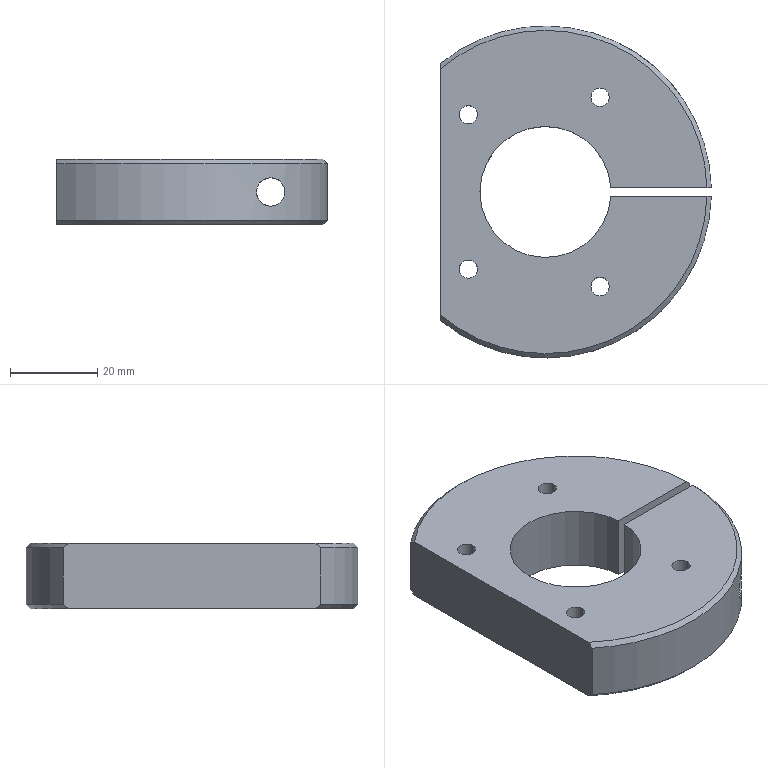Part | SolidWorks | features HoleWzd 3, Chamfer 1, Extrusion 1, ICE 1, RevCut 1 | 1 solid | 28 faces | box 61.987 x 76 x 15 mm | volume 44061 mm3 | cylinder 18 | plane 6 | cone 4 | commonest cylinder face diameters 4.2 x8 6.5 x4 11 x2 30 x2 76 x2
STEP:
#1=CARTESIAN_POINT('',(25.,-28.618,3.25));
#2=VERTEX_POINT('',#1);
#3=CARTESIAN_POINT('',(25.,-28.618,-3.25));
#4=VERTEX_POINT('',#3);
#5=CARTESIAN_POINT('',(25.,-28.618,3.25));
#6=CARTESIAN_POINT('',(24.632,-28.94,3.25));
#7=CARTESIAN_POINT('',(24.265,-29.248,3.189));
#8=CARTESIAN_POINT('',(23.719,-29.69,2.993));
#9=CARTESIAN_POINT('',(23.538,-29.833,2.91));
#10=CARTESIAN_POINT('',(23.192,-30.103,2.708));
#11=CARTESIAN_POINT('',(23.024,-30.231,2.589));
#12=CARTESIAN_POINT('',(22.704,-30.472,2.31));
#13=CARTESIAN_POINT('',(22.554,-30.583,2.152));
#14=CARTESIAN_POINT('',(22.285,-30.78,1.8));
#15=CARTESIAN_POINT('',(22.164,-30.867,1.604));
#16=CARTESIAN_POINT('',(21.965,-31.009,1.184));
#17=CARTESIAN_POINT('',(21.887,-31.064,0.9629));
#18=CARTESIAN_POINT('',(21.806,-31.121,0.6114));
#19=CARTESIAN_POINT('',(21.785,-31.135,0.4903));
#20=CARTESIAN_POINT('',(21.757,-31.155,0.2493));
#21=CARTESIAN_POINT('',(21.75,-31.16,0.1285));
#22=CARTESIAN_POINT('',(21.749,-31.16,-0.2346));
#23=CARTESIAN_POINT('',(21.777,-31.141,-0.481));
#24=CARTESIAN_POINT('',(21.883,-31.067,-0.9495));
#25=CARTESIAN_POINT('',(21.961,-31.012,-1.176));
#26=CARTESIAN_POINT('',(22.161,-30.869,-1.599));
#27=CARTESIAN_POINT('',(22.28,-30.784,-1.793));
#28=CARTESIAN_POINT('',(22.551,-30.585,-2.149));
#29=CARTESIAN_POINT('',(22.701,-30.475,-2.307));
#30=CARTESIAN_POINT('',(23.02,-30.235,-2.586));
#31=CARTESIAN_POINT('',(23.19,-30.104,-2.707));
#32=CARTESIAN_POINT('',(23.538,-29.833,-2.91));
#33=CARTESIAN_POINT('',(23.716,-29.692,-2.992));
#34=CARTESIAN_POINT('',(24.079,-29.399,-3.123));
#35=CARTESIAN_POINT('',(24.265,-29.245,-3.171));
#36=CARTESIAN_POINT('',(24.634,-28.935,-3.235));
#37=CARTESIAN_POINT('',(24.817,-28.778,-3.25));
#38=CARTESIAN_POINT('',(25.,-28.618,-3.25));
#39=B_SPLINE_CURVE_WITH_KNOTS('',3,(#5,#6,#7,#8,#9,#10,#11,#12,#13,#14,#15,#16,#17,#18,#19,#20,#21,#22,#23,#24,#25,#26,#27,#28,#29,#30,#31,#32,#33,#34,#35,#36,#37,#38),.UNSPECIFIED.,.F.,.F.,(4,2,2,2,2,2,2,2,2,2,2,2,2,2,2,2,4),(0.,0.001448,0.002172,0.002897,0.003621,0.004345,0.005069,0.005431,0.005793,0.006517,0.007241,0.007966,0.00869,0.009414,0.01014,0.01086,0.01159),.UNSPECIFIED.);
#40=EDGE_CURVE('',#2,#4,#39,.T.);
#41=ORIENTED_EDGE('',*,*,#40,.T.);
#42=CARTESIAN_POINT('',(25.,-1.,-3.25));
#43=VERTEX_POINT('',#42);
#44=CARTESIAN_POINT('',(25.,32.615,-3.25));
#45=DIRECTION('',(0.,1.,0.));
#46=VECTOR('',#45,1000.);
#47=LINE('',#44,#46);
#48=EDGE_CURVE('',#4,#43,#47,.T.);
#49=ORIENTED_EDGE('',*,*,#48,.T.);
#50=CARTESIAN_POINT('',(25.,-1.,3.25));
#51=VERTEX_POINT('',#50);
#52=CARTESIAN_POINT('',(25.,-1.,0.));
#53=DIRECTION('',(0.,-1.,0.));
#54=DIRECTION('',(1.,0.,0.));
#55=AXIS2_PLACEMENT_3D('',#52,#53,#54);
#56=CIRCLE('',#55,3.25);
#57=EDGE_CURVE('',#51,#43,#56,.T.);
#58=ORIENTED_EDGE('',*,*,#57,.F.);
#59=CARTESIAN_POINT('',(25.,32.615,3.25));
#60=DIRECTION('',(0.,1.,0.));
#61=VECTOR('',#60,1000.);
#62=LINE('',#59,#61);
#63=EDGE_CURVE('',#2,#51,#62,.T.);
#64=ORIENTED_EDGE('',*,*,#63,.F.);
#65=EDGE_LOOP('',(#41,#49,#58,#64));
#66=FACE_OUTER_BOUND('',#65,.T.);
#67=CARTESIAN_POINT('',(25.,32.615,0.));
#68=DIRECTION('',(0.,1.,0.));
#69=DIRECTION('',(0.,0.,1.));
#70=AXIS2_PLACEMENT_3D('',#67,#68,#69);
#71=CYLINDRICAL_SURFACE('',#70,3.25);
#72=ADVANCED_FACE('',(#66),#71,.F.);
#73=CARTESIAN_POINT('',(25.,8.,-5.5));
#74=VERTEX_POINT('',#73);
#75=CARTESIAN_POINT('',(25.,8.,5.5));
#76=VERTEX_POINT('',#75);
#77=CARTESIAN_POINT('',(25.,8.,0.));
#78=DIRECTION('',(0.,1.,0.));
#79=DIRECTION('',(0.,0.,1.));
#80=AXIS2_PLACEMENT_3D('',#77,#78,#79);
#81=CIRCLE('',#80,5.5);
#82=EDGE_CURVE('',#74,#76,#81,.T.);
#83=ORIENTED_EDGE('',*,*,#82,.F.);
#84=CARTESIAN_POINT('',(25.,28.618,-5.5));
#85=VERTEX_POINT('',#84);
#86=CARTESIAN_POINT('',(25.,32.615,-5.5));
#87=DIRECTION('',(0.,1.,0.));
#88=VECTOR('',#87,1000.);
#89=LINE('',#86,#88);
#90=EDGE_CURVE('',#74,#85,#89,.T.);
#91=ORIENTED_EDGE('',*,*,#90,.T.);
#92=CARTESIAN_POINT('',(25.,28.618,5.5));
#93=VERTEX_POINT('',#92);
#94=CARTESIAN_POINT('',(25.,28.618,-5.5));
#95=CARTESIAN_POINT('',(24.694,28.886,-5.5));
#96=CARTESIAN_POINT('',(24.384,29.148,-5.474));
#97=CARTESIAN_POINT('',(23.766,29.654,-5.369));
#98=CARTESIAN_POINT('',(23.457,29.899,-5.289));
#99=CARTESIAN_POINT('',(22.838,30.374,-5.068));
#100=CARTESIAN_POINT('',(22.529,30.603,-4.926));
#101=CARTESIAN_POINT('',(21.937,31.031,-4.581));
#102=CARTESIAN_POINT('',(21.651,31.23,-4.378));
#103=CARTESIAN_POINT('',(21.242,31.509,-4.02));
#104=CARTESIAN_POINT('',(21.109,31.598,-3.892));
#105=CARTESIAN_POINT('',(20.857,31.765,-3.622));
#106=CARTESIAN_POINT('',(20.736,31.844,-3.479));
#107=CARTESIAN_POINT('',(20.509,31.991,-3.18));
#108=CARTESIAN_POINT('',(20.401,32.059,-3.023));
#109=CARTESIAN_POINT('',(20.2,32.186,-2.692));
#110=CARTESIAN_POINT('',(20.107,32.245,-2.519));
#111=CARTESIAN_POINT('',(19.857,32.4,-1.987));
#112=CARTESIAN_POINT('',(19.727,32.479,-1.614));
#113=CARTESIAN_POINT('',(19.593,32.56,-1.025));
#114=CARTESIAN_POINT('',(19.558,32.58,-0.8225));
#115=CARTESIAN_POINT('',(19.512,32.608,-0.4199));
#116=CARTESIAN_POINT('',(19.501,32.615,-0.2183));
#117=CARTESIAN_POINT('',(19.499,32.616,0.1856));
#118=CARTESIAN_POINT('',(19.51,32.609,0.3879));
#119=CARTESIAN_POINT('',(19.554,32.583,0.7932));
#120=CARTESIAN_POINT('',(19.587,32.563,0.9947));
#121=CARTESIAN_POINT('',(19.674,32.511,1.387));
#122=CARTESIAN_POINT('',(19.728,32.478,1.579));
#123=CARTESIAN_POINT('',(19.856,32.4,1.956));
#124=CARTESIAN_POINT('',(19.93,32.354,2.142));
#125=CARTESIAN_POINT('',(20.18,32.199,2.679));
#126=CARTESIAN_POINT('',(20.38,32.074,3.008));
#127=CARTESIAN_POINT('',(20.723,31.853,3.463));
#128=CARTESIAN_POINT('',(20.845,31.773,3.608));
#129=CARTESIAN_POINT('',(21.097,31.606,3.88));
#130=CARTESIAN_POINT('',(21.228,31.518,4.007));
#131=CARTESIAN_POINT('',(21.634,31.242,4.365));
#132=CARTESIAN_POINT('',(21.925,31.039,4.573));
#133=CARTESIAN_POINT('',(22.52,30.61,4.921));
#134=CARTESIAN_POINT('',(22.825,30.384,5.062));
#135=CARTESIAN_POINT('',(23.445,29.908,5.286));
#136=CARTESIAN_POINT('',(23.76,29.659,5.368));
#137=CARTESIAN_POINT('',(24.383,29.149,5.474));
#138=CARTESIAN_POINT('',(24.693,28.886,5.5));
#139=CARTESIAN_POINT('',(25.,28.618,5.5));
#140=B_SPLINE_CURVE_WITH_KNOTS('',3,(#94,#95,#96,#97,#98,#99,#100,#101,#102,#103,#104,#105,#106,#107,#108,#109,#110,#111,#112,#113,#114,#115,#116,#117,#118,#119,#120,#121,#122,#123,#124,#125,#126,#127,#128,#129,#130,#131,#132,#133,#134,#135,#136,#137,#138,#139),.UNSPECIFIED.,.F.,.F.,(4,2,2,2,2,2,2,2,2,2,2,2,2,2,2,2,2,2,2,2,2,2,4),(0.02134,0.02255,0.02376,0.02497,0.02618,0.02679,0.0274,0.028,0.02861,0.02982,0.03042,0.03103,0.03163,0.03224,0.03284,0.03345,0.03466,0.03527,0.03587,0.03708,0.03829,0.0395,0.04072),.UNSPECIFIED.);
#141=EDGE_CURVE('',#85,#93,#140,.T.);
#142=ORIENTED_EDGE('',*,*,#141,.T.);
#143=CARTESIAN_POINT('',(25.,32.615,5.5));
#144=DIRECTION('',(0.,1.,0.));
#145=VECTOR('',#144,1000.);
#146=LINE('',#143,#145);
#147=EDGE_CURVE('',#76,#93,#146,.T.);
#148=ORIENTED_EDGE('',*,*,#147,.F.);
#149=EDGE_LOOP('',(#83,#91,#142,#148));
#150=FACE_OUTER_BOUND('',#149,.T.);
#151=CARTESIAN_POINT('',(25.,32.615,0.));
#152=DIRECTION('',(0.,1.,0.));
#153=DIRECTION('',(0.,0.,1.));
#154=AXIS2_PLACEMENT_3D('',#151,#152,#153);
#155=CYLINDRICAL_SURFACE('',#154,5.5);
#156=ADVANCED_FACE('',(#150),#155,.F.);
#157=CARTESIAN_POINT('',(25.,1.,-3.25));
#158=VERTEX_POINT('',#157);
#159=CARTESIAN_POINT('',(25.,1.,3.25));
#160=VERTEX_POINT('',#159);
#161=CARTESIAN_POINT('',(25.,1.,0.));
#162=DIRECTION('',(0.,1.,0.));
#163=DIRECTION('',(-1.,0.,0.));
#164=AXIS2_PLACEMENT_3D('',#161,#162,#163);
#165=CIRCLE('',#164,3.25);
#166=EDGE_CURVE('',#158,#160,#165,.T.);
#167=ORIENTED_EDGE('',*,*,#166,.F.);
#168=CARTESIAN_POINT('',(25.,8.,-3.25));
#169=VERTEX_POINT('',#168);
#170=CARTESIAN_POINT('',(25.,32.615,-3.25));
#171=DIRECTION('',(0.,1.,0.));
#172=VECTOR('',#171,1000.);
#173=LINE('',#170,#172);
#174=EDGE_CURVE('',#158,#169,#173,.T.);
#175=ORIENTED_EDGE('',*,*,#174,.T.);
#176=CARTESIAN_POINT('',(25.,8.,3.25));
#177=VERTEX_POINT('',#176);
#178=CARTESIAN_POINT('',(25.,8.,0.));
#179=DIRECTION('',(0.,1.,0.));
#180=DIRECTION('',(0.,0.,1.));
#181=AXIS2_PLACEMENT_3D('',#178,#179,#180);
#182=CIRCLE('',#181,3.25);
#183=EDGE_CURVE('',#169,#177,#182,.T.);
#184=ORIENTED_EDGE('',*,*,#183,.T.);
#185=CARTESIAN_POINT('',(25.,32.615,3.25));
#186=DIRECTION('',(0.,1.,0.));
#187=VECTOR('',#186,1000.);
#188=LINE('',#185,#187);
#189=EDGE_CURVE('',#160,#177,#188,.T.);
#190=ORIENTED_EDGE('',*,*,#189,.F.);
#191=EDGE_LOOP('',(#167,#175,#184,#190));
#192=FACE_OUTER_BOUND('',#191,.T.);
#193=CARTESIAN_POINT('',(25.,32.615,0.));
#194=DIRECTION('',(0.,1.,0.));
#195=DIRECTION('',(0.,0.,1.));
#196=AXIS2_PLACEMENT_3D('',#193,#194,#195);
#197=CYLINDRICAL_SURFACE('',#196,3.25);
#198=ADVANCED_FACE('',(#192),#197,.F.);
#199=CARTESIAN_POINT('',(-19.778,-17.678,-7.5));
#200=VERTEX_POINT('',#199);
#201=CARTESIAN_POINT('',(-15.578,-17.678,-7.5));
#202=VERTEX_POINT('',#201);
#203=CARTESIAN_POINT('',(-17.678,-17.678,-7.5));
#204=DIRECTION('',(0.,0.,1.));
#205=DIRECTION('',(1.,0.,0.));
#206=AXIS2_PLACEMENT_3D('',#203,#204,#205);
#207=CIRCLE('',#206,2.1);
#208=EDGE_CURVE('',#200,#202,#207,.T.);
#209=ORIENTED_EDGE('',*,*,#208,.F.);
#210=CARTESIAN_POINT('',(-19.778,-17.678,7.5));
#211=VERTEX_POINT('',#210);
#212=CARTESIAN_POINT('',(-19.778,-17.678,7.5));
#213=DIRECTION('',(0.,0.,1.));
#214=VECTOR('',#213,1000.);
#215=LINE('',#212,#214);
#216=EDGE_CURVE('',#200,#211,#215,.T.);
#217=ORIENTED_EDGE('',*,*,#216,.T.);
#218=CARTESIAN_POINT('',(-15.578,-17.678,7.5));
#219=VERTEX_POINT('',#218);
#220=CARTESIAN_POINT('',(-17.678,-17.678,7.5));
#221=DIRECTION('',(0.,0.,1.));
#222=DIRECTION('',(1.,0.,0.));
#223=AXIS2_PLACEMENT_3D('',#220,#221,#222);
#224=CIRCLE('',#223,2.1);
#225=EDGE_CURVE('',#211,#219,#224,.T.);
#226=ORIENTED_EDGE('',*,*,#225,.T.);
#227=CARTESIAN_POINT('',(-15.578,-17.678,7.5));
#228=DIRECTION('',(0.,0.,1.));
#229=VECTOR('',#228,1000.);
#230=LINE('',#227,#229);
#231=EDGE_CURVE('',#202,#219,#230,.T.);
#232=ORIENTED_EDGE('',*,*,#231,.F.);
#233=EDGE_LOOP('',(#209,#217,#226,#232));
#234=FACE_OUTER_BOUND('',#233,.T.);
#235=CARTESIAN_POINT('',(-17.678,-17.678,7.5));
#236=DIRECTION('',(0.,0.,1.));
#237=DIRECTION('',(1.,0.,0.));
#238=AXIS2_PLACEMENT_3D('',#235,#236,#237);
#239=CYLINDRICAL_SURFACE('',#238,2.1);
#240=ADVANCED_FACE('',(#234),#239,.F.);
#241=CARTESIAN_POINT('',(-19.778,17.678,-7.5));
#242=VERTEX_POINT('',#241);
#243=CARTESIAN_POINT('',(-15.578,17.678,-7.5));
#244=VERTEX_POINT('',#243);
#245=CARTESIAN_POINT('',(-17.678,17.678,-7.5));
#246=DIRECTION('',(0.,0.,1.));
#247=DIRECTION('',(1.,0.,0.));
#248=AXIS2_PLACEMENT_3D('',#245,#246,#247);
#249=CIRCLE('',#248,2.1);
#250=EDGE_CURVE('',#242,#244,#249,.T.);
#251=ORIENTED_EDGE('',*,*,#250,.F.);
#252=CARTESIAN_POINT('',(-19.778,17.678,7.5));
#253=VERTEX_POINT('',#252);
#254=CARTESIAN_POINT('',(-19.778,17.678,7.5));
#255=DIRECTION('',(0.,0.,1.));
#256=VECTOR('',#255,1000.);
#257=LINE('',#254,#256);
#258=EDGE_CURVE('',#242,#253,#257,.T.);
#259=ORIENTED_EDGE('',*,*,#258,.T.);
#260=CARTESIAN_POINT('',(-15.578,17.678,7.5));
#261=VERTEX_POINT('',#260);
#262=CARTESIAN_POINT('',(-17.678,17.678,7.5));
#263=DIRECTION('',(0.,0.,1.));
#264=DIRECTION('',(1.,0.,0.));
#265=AXIS2_PLACEMENT_3D('',#262,#263,#264);
#266=CIRCLE('',#265,2.1);
#267=EDGE_CURVE('',#253,#261,#266,.T.);
#268=ORIENTED_EDGE('',*,*,#267,.T.);
#269=CARTESIAN_POINT('',(-15.578,17.678,7.5));
#270=DIRECTION('',(0.,0.,1.));
#271=VECTOR('',#270,1000.);
#272=LINE('',#269,#271);
#273=EDGE_CURVE('',#244,#261,#272,.T.);
#274=ORIENTED_EDGE('',*,*,#273,.F.);
#275=EDGE_LOOP('',(#251,#259,#268,#274));
#276=FACE_OUTER_BOUND('',#275,.T.);
#277=CARTESIAN_POINT('',(-17.678,17.678,7.5));
#278=DIRECTION('',(0.,0.,1.));
#279=DIRECTION('',(1.,0.,0.));
#280=AXIS2_PLACEMENT_3D('',#277,#278,#279);
#281=CYLINDRICAL_SURFACE('',#280,2.1);
#282=ADVANCED_FACE('',(#276),#281,.F.);
#283=CARTESIAN_POINT('',(10.4,21.651,-7.5));
#284=VERTEX_POINT('',#283);
#285=CARTESIAN_POINT('',(14.6,21.651,-7.5));
#286=VERTEX_POINT('',#285);
#287=CARTESIAN_POINT('',(12.5,21.651,-7.5));
#288=DIRECTION('',(0.,0.,1.));
#289=DIRECTION('',(1.,0.,0.));
#290=AXIS2_PLACEMENT_3D('',#287,#288,#289);
#291=CIRCLE('',#290,2.1);
#292=EDGE_CURVE('',#284,#286,#291,.T.);
#293=ORIENTED_EDGE('',*,*,#292,.F.);
#294=CARTESIAN_POINT('',(10.4,21.651,7.5));
#295=VERTEX_POINT('',#294);
#296=CARTESIAN_POINT('',(10.4,21.651,7.5));
#297=DIRECTION('',(0.,0.,1.));
#298=VECTOR('',#297,1000.);
#299=LINE('',#296,#298);
#300=EDGE_CURVE('',#284,#295,#299,.T.);
#301=ORIENTED_EDGE('',*,*,#300,.T.);
#302=CARTESIAN_POINT('',(14.6,21.651,7.5));
#303=VERTEX_POINT('',#302);
#304=CARTESIAN_POINT('',(12.5,21.651,7.5));
#305=DIRECTION('',(0.,0.,1.));
#306=DIRECTION('',(1.,0.,0.));
#307=AXIS2_PLACEMENT_3D('',#304,#305,#306);
#308=CIRCLE('',#307,2.1);
#309=EDGE_CURVE('',#295,#303,#308,.T.);
#310=ORIENTED_EDGE('',*,*,#309,.T.);
#311=CARTESIAN_POINT('',(14.6,21.651,7.5));
#312=DIRECTION('',(0.,0.,1.));
#313=VECTOR('',#312,1000.);
#314=LINE('',#311,#313);
#315=EDGE_CURVE('',#286,#303,#314,.T.);
#316=ORIENTED_EDGE('',*,*,#315,.F.);
#317=EDGE_LOOP('',(#293,#301,#310,#316));
#318=FACE_OUTER_BOUND('',#317,.T.);
#319=CARTESIAN_POINT('',(12.5,21.651,7.5));
#320=DIRECTION('',(0.,0.,1.));
#321=DIRECTION('',(1.,0.,0.));
#322=AXIS2_PLACEMENT_3D('',#319,#320,#321);
#323=CYLINDRICAL_SURFACE('',#322,2.1);
#324=ADVANCED_FACE('',(#318),#323,.F.);
#325=CARTESIAN_POINT('',(10.4,-21.651,-7.5));
#326=VERTEX_POINT('',#325);
#327=CARTESIAN_POINT('',(14.6,-21.651,-7.5));
#328=VERTEX_POINT('',#327);
#329=CARTESIAN_POINT('',(12.5,-21.651,-7.5));
#330=DIRECTION('',(0.,0.,1.));
#331=DIRECTION('',(1.,0.,0.));
#332=AXIS2_PLACEMENT_3D('',#329,#330,#331);
#333=CIRCLE('',#332,2.1);
#334=EDGE_CURVE('',#326,#328,#333,.T.);
#335=ORIENTED_EDGE('',*,*,#334,.F.);
#336=CARTESIAN_POINT('',(10.4,-21.651,7.5));
#337=VERTEX_POINT('',#336);
#338=CARTESIAN_POINT('',(10.4,-21.651,7.5));
#339=DIRECTION('',(0.,0.,1.));
#340=VECTOR('',#339,1000.);
#341=LINE('',#338,#340);
#342=EDGE_CURVE('',#326,#337,#341,.T.);
#343=ORIENTED_EDGE('',*,*,#342,.T.);
#344=CARTESIAN_POINT('',(14.6,-21.651,7.5));
#345=VERTEX_POINT('',#344);
#346=CARTESIAN_POINT('',(12.5,-21.651,7.5));
#347=DIRECTION('',(0.,0.,1.));
#348=DIRECTION('',(1.,0.,0.));
#349=AXIS2_PLACEMENT_3D('',#346,#347,#348);
#350=CIRCLE('',#349,2.1);
#351=EDGE_CURVE('',#337,#345,#350,.T.);
#352=ORIENTED_EDGE('',*,*,#351,.T.);
#353=CARTESIAN_POINT('',(14.6,-21.651,7.5));
#354=DIRECTION('',(0.,0.,1.));
#355=VECTOR('',#354,1000.);
#356=LINE('',#353,#355);
#357=EDGE_CURVE('',#328,#345,#356,.T.);
#358=ORIENTED_EDGE('',*,*,#357,.F.);
#359=EDGE_LOOP('',(#335,#343,#352,#358));
#360=FACE_OUTER_BOUND('',#359,.T.);
#361=CARTESIAN_POINT('',(12.5,-21.651,7.5));
#362=DIRECTION('',(0.,0.,1.));
#363=DIRECTION('',(1.,0.,0.));
#364=AXIS2_PLACEMENT_3D('',#361,#362,#363);
#365=CYLINDRICAL_SURFACE('',#364,2.1);
#366=ADVANCED_FACE('',(#360),#365,.F.);
#367=CARTESIAN_POINT('',(-15.,0.,7.5));
#368=VERTEX_POINT('',#367);
#369=CARTESIAN_POINT('',(14.967,1.,7.5));
#370=VERTEX_POINT('',#369);
#371=CARTESIAN_POINT('',(0.,0.,7.5));
#372=DIRECTION('',(0.,0.,-1.));
#373=DIRECTION('',(-1.,0.,0.));
#374=AXIS2_PLACEMENT_3D('',#371,#372,#373);
#375=CIRCLE('',#374,15.);
#376=EDGE_CURVE('',#368,#370,#375,.T.);
#377=ORIENTED_EDGE('',*,*,#376,.F.);
#378=CARTESIAN_POINT('',(-15.,0.,-7.5));
#379=VERTEX_POINT('',#378);
#380=CARTESIAN_POINT('',(-15.,0.,7.5));
#381=DIRECTION('',(0.,0.,-1.));
#382=VECTOR('',#381,1000.);
#383=LINE('',#380,#382);
#384=EDGE_CURVE('',#368,#379,#383,.T.);
#385=ORIENTED_EDGE('',*,*,#384,.T.);
#386=CARTESIAN_POINT('',(14.967,1.,-7.5));
#387=VERTEX_POINT('',#386);
#388=CARTESIAN_POINT('',(0.,0.,-7.5));
#389=DIRECTION('',(0.,0.,-1.));
#390=DIRECTION('',(-1.,0.,0.));
#391=AXIS2_PLACEMENT_3D('',#388,#389,#390);
#392=CIRCLE('',#391,15.);
#393=EDGE_CURVE('',#379,#387,#392,.T.);
#394=ORIENTED_EDGE('',*,*,#393,.T.);
#395=CARTESIAN_POINT('',(14.967,1.,-7.5));
#396=DIRECTION('',(0.,0.,1.));
#397=VECTOR('',#396,1000.);
#398=LINE('',#395,#397);
#399=EDGE_CURVE('',#387,#370,#398,.T.);
#400=ORIENTED_EDGE('',*,*,#399,.T.);
#401=EDGE_LOOP('',(#377,#385,#394,#400));
#402=FACE_OUTER_BOUND('',#401,.T.);
#403=CARTESIAN_POINT('',(0.,0.,7.5));
#404=DIRECTION('',(0.,0.,-1.));
#405=DIRECTION('',(-1.,0.,0.));
#406=AXIS2_PLACEMENT_3D('',#403,#404,#405);
#407=CYLINDRICAL_SURFACE('',#406,15.);
#408=ADVANCED_FACE('',(#402),#407,.F.);
#409=ORIENTED_EDGE('',*,*,#40,.F.);
#410=CARTESIAN_POINT('',(25.,-28.618,-3.25));
#411=CARTESIAN_POINT('',(25.193,-28.45,-3.25));
#412=CARTESIAN_POINT('',(25.385,-28.278,-3.233));
#413=CARTESIAN_POINT('',(25.761,-27.936,-3.165));
#414=CARTESIAN_POINT('',(25.945,-27.766,-3.116));
#415=CARTESIAN_POINT('',(26.302,-27.428,-2.984));
#416=CARTESIAN_POINT('',(26.476,-27.259,-2.902));
#417=CARTESIAN_POINT('',(26.815,-26.926,-2.703));
#418=CARTESIAN_POINT('',(26.977,-26.764,-2.587));
#419=CARTESIAN_POINT('',(27.283,-26.452,-2.322));
#420=CARTESIAN_POINT('',(27.426,-26.303,-2.173));
#421=CARTESIAN_POINT('',(27.694,-26.021,-1.831));
#422=CARTESIAN_POINT('',(27.813,-25.893,-1.644));
#423=CARTESIAN_POINT('',(28.018,-25.671,-1.228));
#424=CARTESIAN_POINT('',(28.103,-25.578,-0.9987));
#425=CARTESIAN_POINT('',(28.218,-25.451,-0.5157));
#426=CARTESIAN_POINT('',(28.25,-25.415,-0.2565));
#427=CARTESIAN_POINT('',(28.25,-25.415,0.2546));
#428=CARTESIAN_POINT('',(28.219,-25.45,0.5142));
#429=CARTESIAN_POINT('',(28.103,-25.578,0.9981));
#430=CARTESIAN_POINT('',(28.018,-25.671,1.228));
#431=CARTESIAN_POINT('',(27.814,-25.892,1.642));
#432=CARTESIAN_POINT('',(27.693,-26.022,1.832));
#433=CARTESIAN_POINT('',(27.427,-26.302,2.172));
#434=CARTESIAN_POINT('',(27.284,-26.451,2.321));
#435=CARTESIAN_POINT('',(26.978,-26.763,2.587));
#436=CARTESIAN_POINT('',(26.814,-26.927,2.703));
#437=CARTESIAN_POINT('',(26.477,-27.258,2.901));
#438=CARTESIAN_POINT('',(26.304,-27.426,2.983));
#439=CARTESIAN_POINT('',(25.768,-27.933,3.181));
#440=CARTESIAN_POINT('',(25.388,-28.279,3.25));
#441=CARTESIAN_POINT('',(25.,-28.618,3.25));
#442=B_SPLINE_CURVE_WITH_KNOTS('',3,(#410,#411,#412,#413,#414,#415,#416,#417,#418,#419,#420,#421,#422,#423,#424,#425,#426,#427,#428,#429,#430,#431,#432,#433,#434,#435,#436,#437,#438,#439,#440,#441),.UNSPECIFIED.,.F.,.F.,(4,2,2,2,2,2,2,2,2,2,2,2,2,2,2,4),(0.01159,0.01235,0.01311,0.01388,0.01464,0.01541,0.01617,0.01693,0.0177,0.01846,0.01922,0.01999,0.02075,0.02152,0.02228,0.02381),.UNSPECIFIED.);
#443=EDGE_CURVE('',#4,#2,#442,.T.);
#444=ORIENTED_EDGE('',*,*,#443,.F.);
#445=EDGE_LOOP('',(#409,#444));
#446=FACE_BOUND('',#445,.T.);
#447=CARTESIAN_POINT('',(-24.,-29.462,6.5));
#448=VERTEX_POINT('',#447);
#449=CARTESIAN_POINT('',(-24.,-29.462,-6.5));
#450=VERTEX_POINT('',#449);
#451=CARTESIAN_POINT('',(-24.,-29.462,7.5));
#452=DIRECTION('',(0.,0.,-1.));
#453=VECTOR('',#452,1000.);
#454=LINE('',#451,#453);
#455=EDGE_CURVE('',#448,#450,#454,.T.);
#456=ORIENTED_EDGE('',*,*,#455,.T.);
#457=CARTESIAN_POINT('',(37.987,-1.,-6.5));
#458=VERTEX_POINT('',#457);
#459=CARTESIAN_POINT('',(0.,0.,-6.5));
#460=DIRECTION('',(0.,0.,1.));
#461=DIRECTION('',(-1.,0.,0.));
#462=AXIS2_PLACEMENT_3D('',#459,#460,#461);
#463=CIRCLE('',#462,38.);
#464=EDGE_CURVE('',#450,#458,#463,.T.);
#465=ORIENTED_EDGE('',*,*,#464,.T.);
#466=CARTESIAN_POINT('',(37.987,-1.,6.5));
#467=VERTEX_POINT('',#466);
#468=CARTESIAN_POINT('',(37.987,-1.,-7.5));
#469=DIRECTION('',(0.,0.,1.));
#470=VECTOR('',#469,1000.);
#471=LINE('',#468,#470);
#472=EDGE_CURVE('',#458,#467,#471,.T.);
#473=ORIENTED_EDGE('',*,*,#472,.T.);
#474=CARTESIAN_POINT('',(0.,0.,6.5));
#475=DIRECTION('',(0.,0.,-1.));
#476=DIRECTION('',(-1.,0.,0.));
#477=AXIS2_PLACEMENT_3D('',#474,#475,#476);
#478=CIRCLE('',#477,38.);
#479=EDGE_CURVE('',#467,#448,#478,.T.);
#480=ORIENTED_EDGE('',*,*,#479,.T.);
#481=EDGE_LOOP('',(#456,#465,#473,#480));
#482=FACE_OUTER_BOUND('',#481,.T.);
#483=CARTESIAN_POINT('',(0.,0.,7.5));
#484=DIRECTION('',(0.,0.,-1.));
#485=DIRECTION('',(-1.,0.,0.));
#486=AXIS2_PLACEMENT_3D('',#483,#484,#485);
#487=CYLINDRICAL_SURFACE('',#486,38.);
#488=ADVANCED_FACE('',(#446,#482),#487,.T.);
#489=CARTESIAN_POINT('',(25.,28.618,5.5));
#490=CARTESIAN_POINT('',(25.676,28.027,5.5));
#491=CARTESIAN_POINT('',(26.319,27.424,5.379));
#492=CARTESIAN_POINT('',(27.236,26.503,5.036));
#493=CARTESIAN_POINT('',(27.529,26.197,4.895));
#494=CARTESIAN_POINT('',(28.089,25.597,4.562));
#495=CARTESIAN_POINT('',(28.356,25.3,4.371));
#496=CARTESIAN_POINT('',(28.863,24.72,3.929));
#497=CARTESIAN_POINT('',(29.105,24.433,3.677));
#498=CARTESIAN_POINT('',(29.547,23.897,3.115));
#499=CARTESIAN_POINT('',(29.748,23.647,2.804));
#500=CARTESIAN_POINT('',(30.097,23.2,2.103));
#501=CARTESIAN_POINT('',(30.24,23.012,1.724));
#502=CARTESIAN_POINT('',(30.445,22.741,0.8891));
#503=CARTESIAN_POINT('',(30.5,22.665,0.445));
#504=CARTESIAN_POINT('',(30.5,22.666,-0.2316));
#505=CARTESIAN_POINT('',(30.486,22.685,-0.4537));
#506=CARTESIAN_POINT('',(30.432,22.758,-0.8916));
#507=CARTESIAN_POINT('',(30.391,22.812,-1.109));
#508=CARTESIAN_POINT('',(30.289,22.947,-1.524));
#509=CARTESIAN_POINT('',(30.227,23.029,-1.722));
#510=CARTESIAN_POINT('',(30.086,23.213,-2.104));
#511=CARTESIAN_POINT('',(30.005,23.317,-2.288));
#512=CARTESIAN_POINT('',(29.744,23.651,-2.81));
#513=CARTESIAN_POINT('',(29.544,23.901,-3.119));
#514=CARTESIAN_POINT('',(29.103,24.437,-3.68));
#515=CARTESIAN_POINT('',(28.86,24.723,-3.932));
#516=CARTESIAN_POINT('',(28.353,25.304,-4.373));
#517=CARTESIAN_POINT('',(28.085,25.6,-4.565));
#518=CARTESIAN_POINT('',(27.524,26.203,-4.897));
#519=CARTESIAN_POINT('',(27.228,26.511,-5.039));
#520=CARTESIAN_POINT('',(26.315,27.428,-5.38));
#521=CARTESIAN_POINT('',(25.675,28.029,-5.5));
#522=CARTESIAN_POINT('',(25.,28.618,-5.5));
#523=B_SPLINE_CURVE_WITH_KNOTS('',3,(#489,#490,#491,#492,#493,#494,#495,#496,#497,#498,#499,#500,#501,#502,#503,#504,#505,#506,#507,#508,#509,#510,#511,#512,#513,#514,#515,#516,#517,#518,#519,#520,#521,#522),.UNSPECIFIED.,.F.,.F.,(4,2,2,2,2,2,2,2,2,2,2,2,2,2,2,2,4),(0.,0.002668,0.004001,0.005335,0.006669,0.008003,0.009337,0.01067,0.01134,0.012,0.01267,0.01334,0.01467,0.01601,0.01734,0.01867,0.02134),.UNSPECIFIED.);
#524=EDGE_CURVE('',#93,#85,#523,.T.);
#525=ORIENTED_EDGE('',*,*,#524,.F.);
#526=ORIENTED_EDGE('',*,*,#141,.F.);
#527=EDGE_LOOP('',(#525,#526));
#528=FACE_BOUND('',#527,.T.);
#529=CARTESIAN_POINT('',(-24.,29.462,6.5));
#530=VERTEX_POINT('',#529);
#531=CARTESIAN_POINT('',(-24.,29.462,-6.5));
#532=VERTEX_POINT('',#531);
#533=CARTESIAN_POINT('',(-24.,29.462,7.5));
#534=DIRECTION('',(0.,0.,-1.));
#535=VECTOR('',#534,1000.);
#536=LINE('',#533,#535);
#537=EDGE_CURVE('',#530,#532,#536,.T.);
#538=ORIENTED_EDGE('',*,*,#537,.F.);
#539=CARTESIAN_POINT('',(37.987,1.,6.5));
#540=VERTEX_POINT('',#539);
#541=CARTESIAN_POINT('',(0.,0.,6.5));
#542=DIRECTION('',(0.,0.,-1.));
#543=DIRECTION('',(-1.,0.,0.));
#544=AXIS2_PLACEMENT_3D('',#541,#542,#543);
#545=CIRCLE('',#544,38.);
#546=EDGE_CURVE('',#530,#540,#545,.T.);
#547=ORIENTED_EDGE('',*,*,#546,.T.);
#548=CARTESIAN_POINT('',(37.987,1.,-6.5));
#549=VERTEX_POINT('',#548);
#550=CARTESIAN_POINT('',(37.987,1.,-7.5));
#551=DIRECTION('',(0.,0.,1.));
#552=VECTOR('',#551,1000.);
#553=LINE('',#550,#552);
#554=EDGE_CURVE('',#549,#540,#553,.T.);
#555=ORIENTED_EDGE('',*,*,#554,.F.);
#556=CARTESIAN_POINT('',(0.,0.,-6.5));
#557=DIRECTION('',(0.,0.,1.));
#558=DIRECTION('',(-1.,0.,0.));
#559=AXIS2_PLACEMENT_3D('',#556,#557,#558);
#560=CIRCLE('',#559,38.);
#561=EDGE_CURVE('',#549,#532,#560,.T.);
#562=ORIENTED_EDGE('',*,*,#561,.T.);
#563=EDGE_LOOP('',(#538,#547,#555,#562));
#564=FACE_OUTER_BOUND('',#563,.T.);
#565=CARTESIAN_POINT('',(0.,0.,7.5));
#566=DIRECTION('',(0.,0.,-1.));
#567=DIRECTION('',(-1.,0.,0.));
#568=AXIS2_PLACEMENT_3D('',#565,#566,#567);
#569=CYLINDRICAL_SURFACE('',#568,38.);
#570=ADVANCED_FACE('',(#528,#564),#569,.T.);
#571=CARTESIAN_POINT('',(-24.,-28.16,-7.5));
#572=VERTEX_POINT('',#571);
#573=CARTESIAN_POINT('',(-24.,28.16,-7.5));
#574=VERTEX_POINT('',#573);
#575=CARTESIAN_POINT('',(-24.,-29.462,-7.5));
#576=DIRECTION('',(0.,1.,0.));
#577=VECTOR('',#576,1000.);
#578=LINE('',#575,#577);
#579=EDGE_CURVE('',#572,#574,#578,.T.);
#580=ORIENTED_EDGE('',*,*,#579,.F.);
#581=CARTESIAN_POINT('',(-24.,-28.16,-7.5));
#582=CARTESIAN_POINT('',(-24.,-28.596,-7.169));
#583=CARTESIAN_POINT('',(-24.,-29.029,-6.835));
#584=CARTESIAN_POINT('',(-24.,-29.462,-6.5));
#585=B_SPLINE_CURVE_WITH_KNOTS('',3,(#581,#582,#583,#584),.UNSPECIFIED.,.F.,.F.,(4,4),(0.,0.001641),.UNSPECIFIED.);
#586=EDGE_CURVE('',#572,#450,#585,.T.);
#587=ORIENTED_EDGE('',*,*,#586,.T.);
#588=ORIENTED_EDGE('',*,*,#455,.F.);
#589=CARTESIAN_POINT('',(-24.,-28.16,7.5));
#590=VERTEX_POINT('',#589);
#591=CARTESIAN_POINT('',(-24.,-29.462,6.5));
#592=CARTESIAN_POINT('',(-24.,-29.029,6.835));
#593=CARTESIAN_POINT('',(-24.,-28.596,7.169));
#594=CARTESIAN_POINT('',(-24.,-28.16,7.5));
#595=B_SPLINE_CURVE_WITH_KNOTS('',3,(#591,#592,#593,#594),.UNSPECIFIED.,.F.,.F.,(4,4),(0.,0.001641),.UNSPECIFIED.);
#596=EDGE_CURVE('',#448,#590,#595,.T.);
#597=ORIENTED_EDGE('',*,*,#596,.T.);
#598=CARTESIAN_POINT('',(-24.,28.16,7.5));
#599=VERTEX_POINT('',#598);
#600=CARTESIAN_POINT('',(-24.,-29.462,7.5));
#601=DIRECTION('',(0.,1.,0.));
#602=VECTOR('',#601,1000.);
#603=LINE('',#600,#602);
#604=EDGE_CURVE('',#590,#599,#603,.T.);
#605=ORIENTED_EDGE('',*,*,#604,.T.);
#606=CARTESIAN_POINT('',(-24.,28.16,7.5));
#607=CARTESIAN_POINT('',(-24.,28.596,7.169));
#608=CARTESIAN_POINT('',(-24.,29.029,6.835));
#609=CARTESIAN_POINT('',(-24.,29.462,6.5));
#610=B_SPLINE_CURVE_WITH_KNOTS('',3,(#606,#607,#608,#609),.UNSPECIFIED.,.F.,.F.,(4,4),(0.,0.001641),.UNSPECIFIED.);
#611=EDGE_CURVE('',#599,#530,#610,.T.);
#612=ORIENTED_EDGE('',*,*,#611,.T.);
#613=ORIENTED_EDGE('',*,*,#537,.T.);
#614=CARTESIAN_POINT('',(-24.,29.462,-6.5));
#615=CARTESIAN_POINT('',(-24.,29.029,-6.835));
#616=CARTESIAN_POINT('',(-24.,28.596,-7.169));
#617=CARTESIAN_POINT('',(-24.,28.16,-7.5));
#618=B_SPLINE_CURVE_WITH_KNOTS('',3,(#614,#615,#616,#617),.UNSPECIFIED.,.F.,.F.,(4,4),(0.,0.001641),.UNSPECIFIED.);
#619=EDGE_CURVE('',#532,#574,#618,.T.);
#620=ORIENTED_EDGE('',*,*,#619,.T.);
#621=EDGE_LOOP('',(#580,#587,#588,#597,#605,#612,#613,#620));
#622=FACE_OUTER_BOUND('',#621,.T.);
#623=CARTESIAN_POINT('',(-24.,-29.462,7.5));
#624=DIRECTION('',(-1.,0.,0.));
#625=DIRECTION('',(0.,0.,1.));
#626=AXIS2_PLACEMENT_3D('',#623,#624,#625);
#627=PLANE('',#626);
#628=ADVANCED_FACE('',(#622),#627,.T.);
#629=CARTESIAN_POINT('',(-17.678,-17.678,7.5));
#630=DIRECTION('',(0.,0.,1.));
#631=DIRECTION('',(1.,0.,0.));
#632=AXIS2_PLACEMENT_3D('',#629,#630,#631);
#633=CIRCLE('',#632,2.1);
#634=EDGE_CURVE('',#219,#211,#633,.T.);
#635=ORIENTED_EDGE('',*,*,#634,.F.);
#636=ORIENTED_EDGE('',*,*,#225,.F.);
#637=EDGE_LOOP('',(#635,#636));
#638=FACE_BOUND('',#637,.T.);
#639=CARTESIAN_POINT('',(-17.678,17.678,7.5));
#640=DIRECTION('',(0.,0.,1.));
#641=DIRECTION('',(1.,0.,0.));
#642=AXIS2_PLACEMENT_3D('',#639,#640,#641);
#643=CIRCLE('',#642,2.1);
#644=EDGE_CURVE('',#261,#253,#643,.T.);
#645=ORIENTED_EDGE('',*,*,#644,.F.);
#646=ORIENTED_EDGE('',*,*,#267,.F.);
#647=EDGE_LOOP('',(#645,#646));
#648=FACE_BOUND('',#647,.T.);
#649=CARTESIAN_POINT('',(12.5,21.651,7.5));
#650=DIRECTION('',(0.,0.,1.));
#651=DIRECTION('',(1.,0.,0.));
#652=AXIS2_PLACEMENT_3D('',#649,#650,#651);
#653=CIRCLE('',#652,2.1);
#654=EDGE_CURVE('',#303,#295,#653,.T.);
#655=ORIENTED_EDGE('',*,*,#654,.F.);
#656=ORIENTED_EDGE('',*,*,#309,.F.);
#657=EDGE_LOOP('',(#655,#656));
#658=FACE_BOUND('',#657,.T.);
#659=CARTESIAN_POINT('',(12.5,-21.651,7.5));
#660=DIRECTION('',(0.,0.,1.));
#661=DIRECTION('',(1.,0.,0.));
#662=AXIS2_PLACEMENT_3D('',#659,#660,#661);
#663=CIRCLE('',#662,2.1);
#664=EDGE_CURVE('',#345,#337,#663,.T.);
#665=ORIENTED_EDGE('',*,*,#664,.F.);
#666=ORIENTED_EDGE('',*,*,#351,.F.);
#667=EDGE_LOOP('',(#665,#666));
#668=FACE_BOUND('',#667,.T.);
#669=CARTESIAN_POINT('',(36.986,1.,7.5));
#670=VERTEX_POINT('',#669);
#671=CARTESIAN_POINT('',(37.987,1.,7.5));
#672=DIRECTION('',(-1.,0.,0.));
#673=VECTOR('',#672,1000.);
#674=LINE('',#671,#673);
#675=EDGE_CURVE('',#670,#370,#674,.T.);
#676=ORIENTED_EDGE('',*,*,#675,.F.);
#677=CARTESIAN_POINT('',(0.,0.,7.5));
#678=DIRECTION('',(0.,0.,1.));
#679=DIRECTION('',(-1.,0.,0.));
#680=AXIS2_PLACEMENT_3D('',#677,#678,#679);
#681=CIRCLE('',#680,37.);
#682=EDGE_CURVE('',#670,#599,#681,.T.);
#683=ORIENTED_EDGE('',*,*,#682,.T.);
#684=ORIENTED_EDGE('',*,*,#604,.F.);
#685=CARTESIAN_POINT('',(36.986,-1.,7.5));
#686=VERTEX_POINT('',#685);
#687=CARTESIAN_POINT('',(0.,0.,7.5));
#688=DIRECTION('',(0.,0.,1.));
#689=DIRECTION('',(-1.,0.,0.));
#690=AXIS2_PLACEMENT_3D('',#687,#688,#689);
#691=CIRCLE('',#690,37.);
#692=EDGE_CURVE('',#590,#686,#691,.T.);
#693=ORIENTED_EDGE('',*,*,#692,.T.);
#694=CARTESIAN_POINT('',(14.967,-1.,7.5));
#695=VERTEX_POINT('',#694);
#696=CARTESIAN_POINT('',(14.967,-1.,7.5));
#697=DIRECTION('',(1.,0.,0.));
#698=VECTOR('',#697,1000.);
#699=LINE('',#696,#698);
#700=EDGE_CURVE('',#695,#686,#699,.T.);
#701=ORIENTED_EDGE('',*,*,#700,.F.);
#702=CARTESIAN_POINT('',(0.,0.,7.5));
#703=DIRECTION('',(0.,0.,-1.));
#704=DIRECTION('',(-1.,0.,0.));
#705=AXIS2_PLACEMENT_3D('',#702,#703,#704);
#706=CIRCLE('',#705,15.);
#707=EDGE_CURVE('',#695,#368,#706,.T.);
#708=ORIENTED_EDGE('',*,*,#707,.T.);
#709=ORIENTED_EDGE('',*,*,#376,.T.);
#710=EDGE_LOOP('',(#676,#683,#684,#693,#701,#708,#709));
#711=FACE_OUTER_BOUND('',#710,.T.);
#712=CARTESIAN_POINT('',(0.,0.,7.5));
#713=DIRECTION('',(0.,0.,-1.));
#714=DIRECTION('',(-1.,0.,0.));
#715=AXIS2_PLACEMENT_3D('',#712,#713,#714);
#716=PLANE('',#715);
#717=ADVANCED_FACE('',(#638,#648,#658,#668,#711),#716,.F.);
#718=CARTESIAN_POINT('',(-17.678,-17.678,-7.5));
#719=DIRECTION('',(0.,0.,1.));
#720=DIRECTION('',(1.,0.,0.));
#721=AXIS2_PLACEMENT_3D('',#718,#719,#720);
#722=CIRCLE('',#721,2.1);
#723=EDGE_CURVE('',#202,#200,#722,.T.);
#724=ORIENTED_EDGE('',*,*,#723,.T.);
#725=ORIENTED_EDGE('',*,*,#208,.T.);
#726=EDGE_LOOP('',(#724,#725));
#727=FACE_BOUND('',#726,.T.);
#728=CARTESIAN_POINT('',(-17.678,17.678,-7.5));
#729=DIRECTION('',(0.,0.,1.));
#730=DIRECTION('',(1.,0.,0.));
#731=AXIS2_PLACEMENT_3D('',#728,#729,#730);
#732=CIRCLE('',#731,2.1);
#733=EDGE_CURVE('',#244,#242,#732,.T.);
#734=ORIENTED_EDGE('',*,*,#733,.T.);
#735=ORIENTED_EDGE('',*,*,#250,.T.);
#736=EDGE_LOOP('',(#734,#735));
#737=FACE_BOUND('',#736,.T.);
#738=CARTESIAN_POINT('',(12.5,21.651,-7.5));
#739=DIRECTION('',(0.,0.,1.));
#740=DIRECTION('',(1.,0.,0.));
#741=AXIS2_PLACEMENT_3D('',#738,#739,#740);
#742=CIRCLE('',#741,2.1);
#743=EDGE_CURVE('',#286,#284,#742,.T.);
#744=ORIENTED_EDGE('',*,*,#743,.T.);
#745=ORIENTED_EDGE('',*,*,#292,.T.);
#746=EDGE_LOOP('',(#744,#745));
#747=FACE_BOUND('',#746,.T.);
#748=CARTESIAN_POINT('',(12.5,-21.651,-7.5));
#749=DIRECTION('',(0.,0.,1.));
#750=DIRECTION('',(1.,0.,0.));
#751=AXIS2_PLACEMENT_3D('',#748,#749,#750);
#752=CIRCLE('',#751,2.1);
#753=EDGE_CURVE('',#328,#326,#752,.T.);
#754=ORIENTED_EDGE('',*,*,#753,.T.);
#755=ORIENTED_EDGE('',*,*,#334,.T.);
#756=EDGE_LOOP('',(#754,#755));
#757=FACE_BOUND('',#756,.T.);
#758=CARTESIAN_POINT('',(14.967,-1.,-7.5));
#759=VERTEX_POINT('',#758);
#760=CARTESIAN_POINT('',(36.986,-1.,-7.5));
#761=VERTEX_POINT('',#760);
#762=CARTESIAN_POINT('',(14.967,-1.,-7.5));
#763=DIRECTION('',(1.,0.,0.));
#764=VECTOR('',#763,1000.);
#765=LINE('',#762,#764);
#766=EDGE_CURVE('',#759,#761,#765,.T.);
#767=ORIENTED_EDGE('',*,*,#766,.T.);
#768=CARTESIAN_POINT('',(0.,0.,-7.5));
#769=DIRECTION('',(0.,0.,-1.));
#770=DIRECTION('',(-1.,0.,0.));
#771=AXIS2_PLACEMENT_3D('',#768,#769,#770);
#772=CIRCLE('',#771,37.);
#773=EDGE_CURVE('',#761,#572,#772,.T.);
#774=ORIENTED_EDGE('',*,*,#773,.T.);
#775=ORIENTED_EDGE('',*,*,#579,.T.);
#776=CARTESIAN_POINT('',(36.986,1.,-7.5));
#777=VERTEX_POINT('',#776);
#778=CARTESIAN_POINT('',(0.,0.,-7.5));
#779=DIRECTION('',(0.,0.,-1.));
#780=DIRECTION('',(-1.,0.,0.));
#781=AXIS2_PLACEMENT_3D('',#778,#779,#780);
#782=CIRCLE('',#781,37.);
#783=EDGE_CURVE('',#574,#777,#782,.T.);
#784=ORIENTED_EDGE('',*,*,#783,.T.);
#785=CARTESIAN_POINT('',(37.987,1.,-7.5));
#786=DIRECTION('',(-1.,0.,0.));
#787=VECTOR('',#786,1000.);
#788=LINE('',#785,#787);
#789=EDGE_CURVE('',#777,#387,#788,.T.);
#790=ORIENTED_EDGE('',*,*,#789,.T.);
#791=ORIENTED_EDGE('',*,*,#393,.F.);
#792=CARTESIAN_POINT('',(0.,0.,-7.5));
#793=DIRECTION('',(0.,0.,-1.));
#794=DIRECTION('',(-1.,0.,0.));
#795=AXIS2_PLACEMENT_3D('',#792,#793,#794);
#796=CIRCLE('',#795,15.);
#797=EDGE_CURVE('',#759,#379,#796,.T.);
#798=ORIENTED_EDGE('',*,*,#797,.F.);
#799=EDGE_LOOP('',(#767,#774,#775,#784,#790,#791,#798));
#800=FACE_OUTER_BOUND('',#799,.T.);
#801=CARTESIAN_POINT('',(0.,0.,-7.5));
#802=DIRECTION('',(0.,0.,-1.));
#803=DIRECTION('',(-1.,0.,0.));
#804=AXIS2_PLACEMENT_3D('',#801,#802,#803);
#805=PLANE('',#804);
#806=ADVANCED_FACE('',(#727,#737,#747,#757,#800),#805,.T.);
#807=ORIENTED_EDGE('',*,*,#57,.T.);
#808=CARTESIAN_POINT('',(25.,-1.,0.));
#809=DIRECTION('',(0.,-1.,0.));
#810=DIRECTION('',(1.,0.,0.));
#811=AXIS2_PLACEMENT_3D('',#808,#809,#810);
#812=CIRCLE('',#811,3.25);
#813=EDGE_CURVE('',#43,#51,#812,.T.);
#814=ORIENTED_EDGE('',*,*,#813,.T.);
#815=EDGE_LOOP('',(#807,#814));
#816=FACE_BOUND('',#815,.T.);
#817=ORIENTED_EDGE('',*,*,#472,.F.);
#818=CARTESIAN_POINT('',(37.987,-1.,-6.5));
#819=CARTESIAN_POINT('',(37.653,-1.,-6.833));
#820=CARTESIAN_POINT('',(37.32,-1.,-7.167));
#821=CARTESIAN_POINT('',(36.986,-1.,-7.5));
#822=B_SPLINE_CURVE_WITH_KNOTS('',3,(#818,#819,#820,#821),.UNSPECIFIED.,.F.,.F.,(4,4),(0.,0.001414),.UNSPECIFIED.);
#823=EDGE_CURVE('',#458,#761,#822,.T.);
#824=ORIENTED_EDGE('',*,*,#823,.T.);
#825=ORIENTED_EDGE('',*,*,#766,.F.);
#826=CARTESIAN_POINT('',(14.967,-1.,-7.5));
#827=DIRECTION('',(0.,0.,1.));
#828=VECTOR('',#827,1000.);
#829=LINE('',#826,#828);
#830=EDGE_CURVE('',#759,#695,#829,.T.);
#831=ORIENTED_EDGE('',*,*,#830,.T.);
#832=ORIENTED_EDGE('',*,*,#700,.T.);
#833=CARTESIAN_POINT('',(36.986,-1.,7.5));
#834=CARTESIAN_POINT('',(37.32,-1.,7.167));
#835=CARTESIAN_POINT('',(37.653,-1.,6.833));
#836=CARTESIAN_POINT('',(37.987,-1.,6.5));
#837=B_SPLINE_CURVE_WITH_KNOTS('',3,(#833,#834,#835,#836),.UNSPECIFIED.,.F.,.F.,(4,4),(0.,0.001414),.UNSPECIFIED.);
#838=EDGE_CURVE('',#686,#467,#837,.T.);
#839=ORIENTED_EDGE('',*,*,#838,.T.);
#840=EDGE_LOOP('',(#817,#824,#825,#831,#832,#839));
#841=FACE_OUTER_BOUND('',#840,.T.);
#842=CARTESIAN_POINT('',(14.967,-1.,-7.5));
#843=DIRECTION('',(0.,-1.,0.));
#844=DIRECTION('',(1.,0.,0.));
#845=AXIS2_PLACEMENT_3D('',#842,#843,#844);
#846=PLANE('',#845);
#847=ADVANCED_FACE('',(#816,#841),#846,.F.);
#848=CARTESIAN_POINT('',(25.,1.,0.));
#849=DIRECTION('',(0.,1.,0.));
#850=DIRECTION('',(-1.,0.,0.));
#851=AXIS2_PLACEMENT_3D('',#848,#849,#850);
#852=CIRCLE('',#851,3.25);
#853=EDGE_CURVE('',#160,#158,#852,.T.);
#854=ORIENTED_EDGE('',*,*,#853,.T.);
#855=ORIENTED_EDGE('',*,*,#166,.T.);
#856=EDGE_LOOP('',(#854,#855));
#857=FACE_BOUND('',#856,.T.);
#858=ORIENTED_EDGE('',*,*,#554,.T.);
#859=CARTESIAN_POINT('',(37.987,1.,6.5));
#860=CARTESIAN_POINT('',(37.653,1.,6.833));
#861=CARTESIAN_POINT('',(37.32,1.,7.167));
#862=CARTESIAN_POINT('',(36.986,1.,7.5));
#863=B_SPLINE_CURVE_WITH_KNOTS('',3,(#859,#860,#861,#862),.UNSPECIFIED.,.F.,.F.,(4,4),(0.,0.001414),.UNSPECIFIED.);
#864=EDGE_CURVE('',#540,#670,#863,.T.);
#865=ORIENTED_EDGE('',*,*,#864,.T.);
#866=ORIENTED_EDGE('',*,*,#675,.T.);
#867=ORIENTED_EDGE('',*,*,#399,.F.);
#868=ORIENTED_EDGE('',*,*,#789,.F.);
#869=CARTESIAN_POINT('',(36.986,1.,-7.5));
#870=CARTESIAN_POINT('',(37.32,1.,-7.167));
#871=CARTESIAN_POINT('',(37.653,1.,-6.833));
#872=CARTESIAN_POINT('',(37.987,1.,-6.5));
#873=B_SPLINE_CURVE_WITH_KNOTS('',3,(#869,#870,#871,#872),.UNSPECIFIED.,.F.,.F.,(4,4),(0.,0.001414),.UNSPECIFIED.);
#874=EDGE_CURVE('',#777,#549,#873,.T.);
#875=ORIENTED_EDGE('',*,*,#874,.T.);
#876=EDGE_LOOP('',(#858,#865,#866,#867,#868,#875));
#877=FACE_OUTER_BOUND('',#876,.T.);
#878=CARTESIAN_POINT('',(37.987,1.,-7.5));
#879=DIRECTION('',(0.,1.,0.));
#880=DIRECTION('',(-1.,0.,0.));
#881=AXIS2_PLACEMENT_3D('',#878,#879,#880);
#882=PLANE('',#881);
#883=ADVANCED_FACE('',(#857,#877),#882,.F.);
#884=ORIENTED_EDGE('',*,*,#384,.F.);
#885=ORIENTED_EDGE('',*,*,#707,.F.);
#886=ORIENTED_EDGE('',*,*,#830,.F.);
#887=ORIENTED_EDGE('',*,*,#797,.T.);
#888=EDGE_LOOP('',(#884,#885,#886,#887));
#889=FACE_OUTER_BOUND('',#888,.T.);
#890=CARTESIAN_POINT('',(0.,0.,7.5));
#891=DIRECTION('',(0.,0.,-1.));
#892=DIRECTION('',(-1.,0.,0.));
#893=AXIS2_PLACEMENT_3D('',#890,#891,#892);
#894=CYLINDRICAL_SURFACE('',#893,15.);
#895=ADVANCED_FACE('',(#889),#894,.F.);
#896=ORIENTED_EDGE('',*,*,#342,.F.);
#897=ORIENTED_EDGE('',*,*,#753,.F.);
#898=ORIENTED_EDGE('',*,*,#357,.T.);
#899=ORIENTED_EDGE('',*,*,#664,.T.);
#900=EDGE_LOOP('',(#896,#897,#898,#899));
#901=FACE_OUTER_BOUND('',#900,.T.);
#902=CARTESIAN_POINT('',(12.5,-21.651,7.5));
#903=DIRECTION('',(0.,0.,1.));
#904=DIRECTION('',(1.,0.,0.));
#905=AXIS2_PLACEMENT_3D('',#902,#903,#904);
#906=CYLINDRICAL_SURFACE('',#905,2.1);
#907=ADVANCED_FACE('',(#901),#906,.F.);
#908=ORIENTED_EDGE('',*,*,#300,.F.);
#909=ORIENTED_EDGE('',*,*,#743,.F.);
#910=ORIENTED_EDGE('',*,*,#315,.T.);
#911=ORIENTED_EDGE('',*,*,#654,.T.);
#912=EDGE_LOOP('',(#908,#909,#910,#911));
#913=FACE_OUTER_BOUND('',#912,.T.);
#914=CARTESIAN_POINT('',(12.5,21.651,7.5));
#915=DIRECTION('',(0.,0.,1.));
#916=DIRECTION('',(1.,0.,0.));
#917=AXIS2_PLACEMENT_3D('',#914,#915,#916);
#918=CYLINDRICAL_SURFACE('',#917,2.1);
#919=ADVANCED_FACE('',(#913),#918,.F.);
#920=ORIENTED_EDGE('',*,*,#258,.F.);
#921=ORIENTED_EDGE('',*,*,#733,.F.);
#922=ORIENTED_EDGE('',*,*,#273,.T.);
#923=ORIENTED_EDGE('',*,*,#644,.T.);
#924=EDGE_LOOP('',(#920,#921,#922,#923));
#925=FACE_OUTER_BOUND('',#924,.T.);
#926=CARTESIAN_POINT('',(-17.678,17.678,7.5));
#927=DIRECTION('',(0.,0.,1.));
#928=DIRECTION('',(1.,0.,0.));
#929=AXIS2_PLACEMENT_3D('',#926,#927,#928);
#930=CYLINDRICAL_SURFACE('',#929,2.1);
#931=ADVANCED_FACE('',(#925),#930,.F.);
#932=ORIENTED_EDGE('',*,*,#216,.F.);
#933=ORIENTED_EDGE('',*,*,#723,.F.);
#934=ORIENTED_EDGE('',*,*,#231,.T.);
#935=ORIENTED_EDGE('',*,*,#634,.T.);
#936=EDGE_LOOP('',(#932,#933,#934,#935));
#937=FACE_OUTER_BOUND('',#936,.T.);
#938=CARTESIAN_POINT('',(-17.678,-17.678,7.5));
#939=DIRECTION('',(0.,0.,1.));
#940=DIRECTION('',(1.,0.,0.));
#941=AXIS2_PLACEMENT_3D('',#938,#939,#940);
#942=CYLINDRICAL_SURFACE('',#941,2.1);
#943=ADVANCED_FACE('',(#937),#942,.F.);
#944=ORIENTED_EDGE('',*,*,#174,.F.);
#945=ORIENTED_EDGE('',*,*,#853,.F.);
#946=ORIENTED_EDGE('',*,*,#189,.T.);
#947=CARTESIAN_POINT('',(25.,8.,0.));
#948=DIRECTION('',(0.,1.,0.));
#949=DIRECTION('',(0.,0.,1.));
#950=AXIS2_PLACEMENT_3D('',#947,#948,#949);
#951=CIRCLE('',#950,3.25);
#952=EDGE_CURVE('',#177,#169,#951,.T.);
#953=ORIENTED_EDGE('',*,*,#952,.T.);
#954=EDGE_LOOP('',(#944,#945,#946,#953));
#955=FACE_OUTER_BOUND('',#954,.T.);
#956=CARTESIAN_POINT('',(25.,32.615,0.));
#957=DIRECTION('',(0.,1.,0.));
#958=DIRECTION('',(0.,0.,1.));
#959=AXIS2_PLACEMENT_3D('',#956,#957,#958);
#960=CYLINDRICAL_SURFACE('',#959,3.25);
#961=ADVANCED_FACE('',(#955),#960,.F.);
#962=ORIENTED_EDGE('',*,*,#952,.F.);
#963=ORIENTED_EDGE('',*,*,#183,.F.);
#964=EDGE_LOOP('',(#962,#963));
#965=FACE_BOUND('',#964,.T.);
#966=CARTESIAN_POINT('',(25.,8.,0.));
#967=DIRECTION('',(0.,1.,0.));
#968=DIRECTION('',(0.,0.,1.));
#969=AXIS2_PLACEMENT_3D('',#966,#967,#968);
#970=CIRCLE('',#969,5.5);
#971=EDGE_CURVE('',#76,#74,#970,.T.);
#972=ORIENTED_EDGE('',*,*,#971,.T.);
#973=ORIENTED_EDGE('',*,*,#82,.T.);
#974=EDGE_LOOP('',(#972,#973));
#975=FACE_OUTER_BOUND('',#974,.T.);
#976=CARTESIAN_POINT('',(28.25,8.,0.));
#977=DIRECTION('',(0.,-1.,0.));
#978=DIRECTION('',(0.,0.,-1.));
#979=AXIS2_PLACEMENT_3D('',#976,#977,#978);
#980=PLANE('',#979);
#981=ADVANCED_FACE('',(#965,#975),#980,.F.);
#982=ORIENTED_EDGE('',*,*,#90,.F.);
#983=ORIENTED_EDGE('',*,*,#971,.F.);
#984=ORIENTED_EDGE('',*,*,#147,.T.);
#985=ORIENTED_EDGE('',*,*,#524,.T.);
#986=EDGE_LOOP('',(#982,#983,#984,#985));
#987=FACE_OUTER_BOUND('',#986,.T.);
#988=CARTESIAN_POINT('',(25.,32.615,0.));
#989=DIRECTION('',(0.,1.,0.));
#990=DIRECTION('',(0.,0.,1.));
#991=AXIS2_PLACEMENT_3D('',#988,#989,#990);
#992=CYLINDRICAL_SURFACE('',#991,5.5);
#993=ADVANCED_FACE('',(#987),#992,.F.);
#994=ORIENTED_EDGE('',*,*,#48,.F.);
#995=ORIENTED_EDGE('',*,*,#443,.T.);
#996=ORIENTED_EDGE('',*,*,#63,.T.);
#997=ORIENTED_EDGE('',*,*,#813,.F.);
#998=EDGE_LOOP('',(#994,#995,#996,#997));
#999=FACE_OUTER_BOUND('',#998,.T.);
#1000=CARTESIAN_POINT('',(25.,32.615,0.));
#1001=DIRECTION('',(0.,1.,0.));
#1002=DIRECTION('',(0.,0.,1.));
#1003=AXIS2_PLACEMENT_3D('',#1000,#1001,#1002);
#1004=CYLINDRICAL_SURFACE('',#1003,3.25);
#1005=ADVANCED_FACE('',(#999),#1004,.F.);
#1006=ORIENTED_EDGE('',*,*,#823,.F.);
#1007=ORIENTED_EDGE('',*,*,#464,.F.);
#1008=ORIENTED_EDGE('',*,*,#586,.F.);
#1009=ORIENTED_EDGE('',*,*,#773,.F.);
#1010=EDGE_LOOP('',(#1006,#1007,#1008,#1009));
#1011=FACE_OUTER_BOUND('',#1010,.T.);
#1012=CARTESIAN_POINT('',(0.,0.,-7.5));
#1013=DIRECTION('',(0.,0.,1.));
#1014=DIRECTION('',(1.,0.,0.));
#1015=AXIS2_PLACEMENT_3D('',#1012,#1013,#1014);
#1016=CONICAL_SURFACE('',#1015,37.,0.7854);
#1017=ADVANCED_FACE('',(#1011),#1016,.T.);
#1018=ORIENTED_EDGE('',*,*,#611,.F.);
#1019=ORIENTED_EDGE('',*,*,#682,.F.);
#1020=ORIENTED_EDGE('',*,*,#864,.F.);
#1021=ORIENTED_EDGE('',*,*,#546,.F.);
#1022=EDGE_LOOP('',(#1018,#1019,#1020,#1021));
#1023=FACE_OUTER_BOUND('',#1022,.T.);
#1024=CARTESIAN_POINT('',(0.,0.,6.5));
#1025=DIRECTION('',(0.,0.,-1.));
#1026=DIRECTION('',(-1.,0.,0.));
#1027=AXIS2_PLACEMENT_3D('',#1024,#1025,#1026);
#1028=CONICAL_SURFACE('',#1027,38.,0.7854);
#1029=ADVANCED_FACE('',(#1023),#1028,.T.);
#1030=ORIENTED_EDGE('',*,*,#619,.F.);
#1031=ORIENTED_EDGE('',*,*,#561,.F.);
#1032=ORIENTED_EDGE('',*,*,#874,.F.);
#1033=ORIENTED_EDGE('',*,*,#783,.F.);
#1034=EDGE_LOOP('',(#1030,#1031,#1032,#1033));
#1035=FACE_OUTER_BOUND('',#1034,.T.);
#1036=CARTESIAN_POINT('',(0.,0.,-7.5));
#1037=DIRECTION('',(0.,0.,1.));
#1038=DIRECTION('',(1.,0.,0.));
#1039=AXIS2_PLACEMENT_3D('',#1036,#1037,#1038);
#1040=CONICAL_SURFACE('',#1039,37.,0.7854);
#1041=ADVANCED_FACE('',(#1035),#1040,.T.);
#1042=ORIENTED_EDGE('',*,*,#838,.F.);
#1043=ORIENTED_EDGE('',*,*,#692,.F.);
#1044=ORIENTED_EDGE('',*,*,#596,.F.);
#1045=ORIENTED_EDGE('',*,*,#479,.F.);
#1046=EDGE_LOOP('',(#1042,#1043,#1044,#1045));
#1047=FACE_OUTER_BOUND('',#1046,.T.);
#1048=CARTESIAN_POINT('',(0.,0.,6.5));
#1049=DIRECTION('',(0.,0.,-1.));
#1050=DIRECTION('',(-1.,0.,0.));
#1051=AXIS2_PLACEMENT_3D('',#1048,#1049,#1050);
#1052=CONICAL_SURFACE('',#1051,38.,0.7854);
#1053=ADVANCED_FACE('',(#1047),#1052,.T.);
#1054=CLOSED_SHELL('',(#72,#156,#198,#240,#282,#324,#366,#408,#488,#570,#628,#717,#806,#847,#883,#895,#907,#919,#931,#943,#961,#981,#993,#1005,#1017,#1029,#1041,#1053));
#1055=MANIFOLD_SOLID_BREP('',#1054);
#1056=CARTESIAN_POINT('',(0.,0.,0.));
#1057=DIRECTION('',(0.,0.,1.));
#1058=DIRECTION('',(1.,0.,0.));
#1059=AXIS2_PLACEMENT_3D('',#1056,#1057,#1058);
#1060=(LENGTH_UNIT()NAMED_UNIT(*)SI_UNIT(.MILLI.,.METRE.));
#1061=UNCERTAINTY_MEASURE_WITH_UNIT(LENGTH_MEASURE(0.00001),#1060,'','');
#1062=(NAMED_UNIT(*)PLANE_ANGLE_UNIT()SI_UNIT($,.RADIAN.));
#1063=(NAMED_UNIT(*)SI_UNIT($,.STERADIAN.)SOLID_ANGLE_UNIT());
#1064=(GEOMETRIC_REPRESENTATION_CONTEXT(3)GLOBAL_UNCERTAINTY_ASSIGNED_CONTEXT((#1061))GLOBAL_UNIT_ASSIGNED_CONTEXT((#1060,#1062,#1063))REPRESENTATION_CONTEXT('',''));
#1065=ADVANCED_BREP_SHAPE_REPRESENTATION('',(#1055,#1059),#1064);